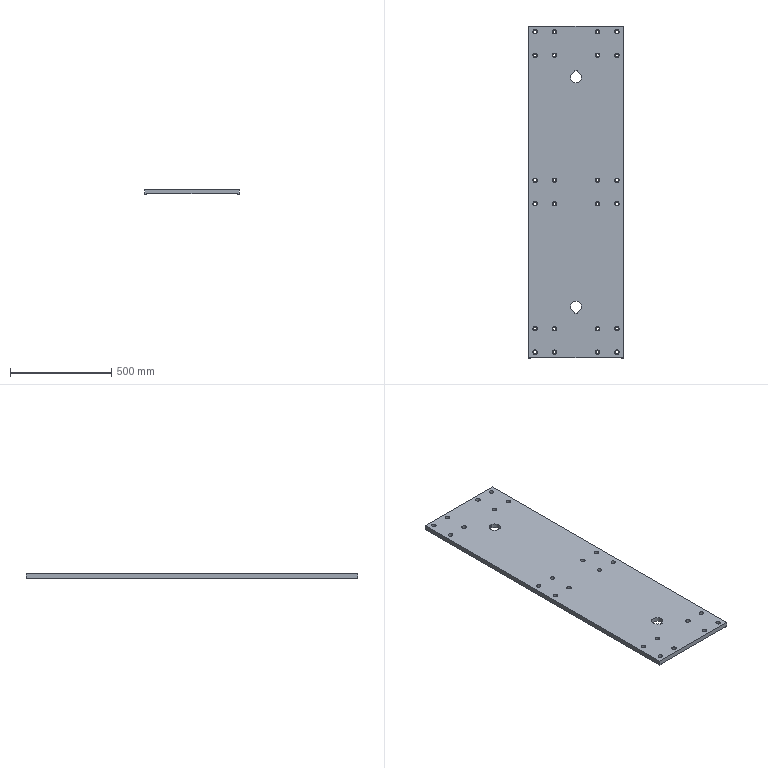Part | Creo | features CURVE 4, DATUM PLANE 3, CUT 2, PROTRUSION 2, COORDINATE SYSTEM 1 | 1 solid | 141 faces | box 468 x 1636 x 24 mm | volume 15910357 mm3 | cylinder 100 | plane 41 | commonest cylinder face diameters 15 x48 22 x48 8.5 x2 55 x2